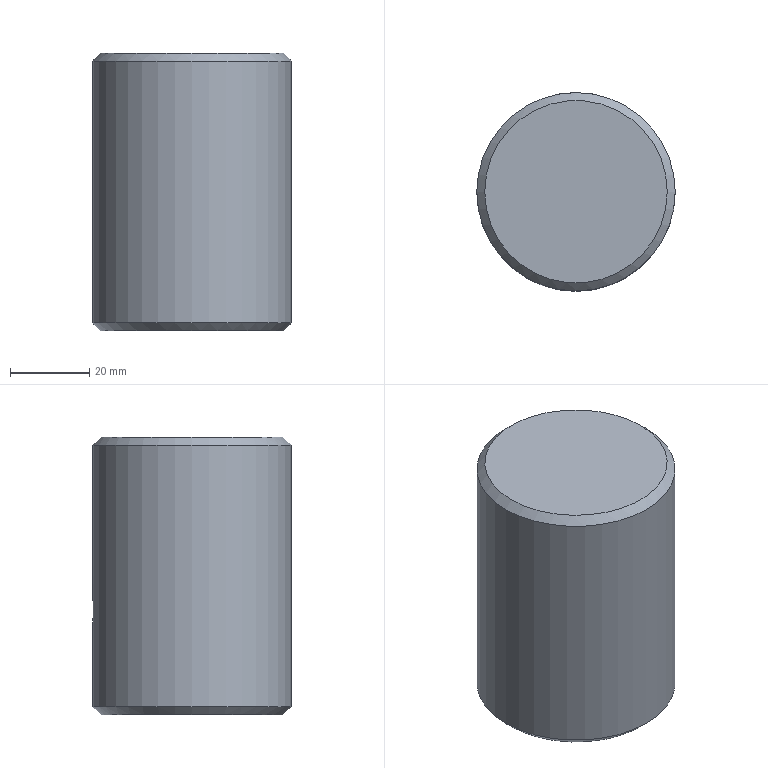Part | NX | features LIN_SOLID_COLOR 2 | 1 solid | 9 faces | box 50 x 50 x 70 mm | volume 134795 mm3 | cone 4 | cylinder 3 | plane 2 | commonest cylinder face diameters 5.2 x1 8.499 x1 50 x1
STEP:
#1=CARTESIAN_POINT('',(609.,370.,-46.5));
#2=VERTEX_POINT('',#1);
#3=CARTESIAN_POINT('',(586.,370.,-46.5));
#4=DIRECTION('',(0.,0.,-1.));
#5=DIRECTION('',(1.,0.,0.));
#6=AXIS2_PLACEMENT_3D('',#3,#4,#5);
#7=CIRCLE('',#6,23.);
#8=EDGE_CURVE('',#2,#2,#7,.T.);
#9=ORIENTED_EDGE('',*,*,#8,.T.);
#10=EDGE_LOOP('',(#9));
#11=FACE_BOUND('',#10,.T.);
#12=CARTESIAN_POINT('',(590.25,370.,-46.5));
#13=VERTEX_POINT('',#12);
#14=CARTESIAN_POINT('',(586.,370.,-46.5));
#15=DIRECTION('',(0.,0.,1.));
#16=DIRECTION('',(1.,0.,0.));
#17=AXIS2_PLACEMENT_3D('',#14,#15,#16);
#18=CIRCLE('',#17,4.25);
#19=EDGE_CURVE('',#13,#13,#18,.T.);
#20=ORIENTED_EDGE('',*,*,#19,.T.);
#21=EDGE_LOOP('',(#20));
#22=FACE_BOUND('',#21,.T.);
#23=CARTESIAN_POINT('',(586.,370.,-46.5));
#24=DIRECTION('',(0.,0.,-1.));
#25=DIRECTION('',(1.,0.,0.));
#26=AXIS2_PLACEMENT_3D('',#23,#24,#25);
#27=PLANE('',#26);
#28=ADVANCED_FACE('',(#11,#22),#27,.T.);
#29=CARTESIAN_POINT('',(563.,370.,23.5));
#30=VERTEX_POINT('',#29);
#31=CARTESIAN_POINT('',(586.,370.,23.5));
#32=DIRECTION('',(0.,0.,1.));
#33=DIRECTION('',(-1.,0.,0.));
#34=AXIS2_PLACEMENT_3D('',#31,#32,#33);
#35=CIRCLE('',#34,23.);
#36=EDGE_CURVE('',#30,#30,#35,.T.);
#37=ORIENTED_EDGE('',*,*,#36,.T.);
#38=EDGE_LOOP('',(#37));
#39=FACE_BOUND('',#38,.T.);
#40=CARTESIAN_POINT('',(586.,370.,23.5));
#41=DIRECTION('',(0.,0.,1.));
#42=DIRECTION('',(-1.,0.,0.));
#43=AXIS2_PLACEMENT_3D('',#40,#41,#42);
#44=PLANE('',#43);
#45=ADVANCED_FACE('',(#39),#44,.T.);
#46=CARTESIAN_POINT('',(588.6,394.864,-20.));
#47=VERTEX_POINT('',#46);
#48=CARTESIAN_POINT('',(588.036,394.933,-17.96));
#49=CARTESIAN_POINT('',(588.882,394.83,-20.001));
#50=CARTESIAN_POINT('',(588.036,394.932,-22.038));
#51=CARTESIAN_POINT('',(586.002,395.034,-22.881));
#52=CARTESIAN_POINT('',(583.963,394.932,-22.039));
#53=CARTESIAN_POINT('',(583.119,394.83,-20.001));
#54=CARTESIAN_POINT('',(583.961,394.932,-17.965));
#55=CARTESIAN_POINT('',(585.997,395.034,-17.119));
#56=CARTESIAN_POINT('',(588.036,394.933,-17.96));
#57=CARTESIAN_POINT('',(588.882,394.83,-20.001));
#58=CARTESIAN_POINT('',(588.036,394.932,-22.038));
#59=B_SPLINE_CURVE_WITH_KNOTS('',3,(#48,#49,#50,#51,#52,#53,#54,#55,#56,#57,#58),.UNSPECIFIED.,.T.,.F.,(1,1,1,1,1,1,1,1,1,1,1,1,1,1,1),(-0.0061,-0.004067,-0.002033,0.,0.002033,0.004067,0.0061,0.008133,0.01017,0.0122,0.01423,0.01627,0.0183,0.02033,0.02237),.UNSPECIFIED.);
#60=EDGE_CURVE('',#47,#47,#59,.T.);
#61=ORIENTED_EDGE('',*,*,#60,.F.);
#62=EDGE_LOOP('',(#61));
#63=FACE_BOUND('',#62,.T.);
#64=CARTESIAN_POINT('',(611.,370.,-44.5));
#65=VERTEX_POINT('',#64);
#66=CARTESIAN_POINT('',(586.,370.,-44.5));
#67=DIRECTION('',(0.,0.,-1.));
#68=DIRECTION('',(1.,0.,0.));
#69=AXIS2_PLACEMENT_3D('',#66,#67,#68);
#70=CIRCLE('',#69,25.);
#71=EDGE_CURVE('',#65,#65,#70,.F.);
#72=ORIENTED_EDGE('',*,*,#71,.T.);
#73=EDGE_LOOP('',(#72));
#74=FACE_BOUND('',#73,.T.);
#75=CARTESIAN_POINT('',(561.,370.,21.5));
#76=VERTEX_POINT('',#75);
#77=CARTESIAN_POINT('',(586.,370.,21.5));
#78=DIRECTION('',(0.,0.,1.));
#79=DIRECTION('',(-1.,0.,0.));
#80=AXIS2_PLACEMENT_3D('',#77,#78,#79);
#81=CIRCLE('',#80,25.);
#82=EDGE_CURVE('',#76,#76,#81,.F.);
#83=ORIENTED_EDGE('',*,*,#82,.T.);
#84=EDGE_LOOP('',(#83));
#85=FACE_BOUND('',#84,.T.);
#86=CARTESIAN_POINT('',(586.,370.,3.5));
#87=DIRECTION('',(0.,0.,-1.));
#88=DIRECTION('',(1.,0.,0.));
#89=AXIS2_PLACEMENT_3D('',#86,#87,#88);
#90=CYLINDRICAL_SURFACE('',#89,25.);
#91=ADVANCED_FACE('',(#63,#74,#85),#90,.T.);
#92=ORIENTED_EDGE('',*,*,#71,.F.);
#93=EDGE_LOOP('',(#92));
#94=FACE_BOUND('',#93,.T.);
#95=ORIENTED_EDGE('',*,*,#8,.F.);
#96=EDGE_LOOP('',(#95));
#97=FACE_BOUND('',#96,.T.);
#98=CARTESIAN_POINT('',(586.,370.,-46.5));
#99=DIRECTION('',(0.,0.,1.));
#100=DIRECTION('',(-1.,0.,0.));
#101=AXIS2_PLACEMENT_3D('',#98,#99,#100);
#102=CONICAL_SURFACE('',#101,23.,0.7854);
#103=ADVANCED_FACE('',(#94,#97),#102,.T.);
#104=ORIENTED_EDGE('',*,*,#36,.F.);
#105=EDGE_LOOP('',(#104));
#106=FACE_BOUND('',#105,.T.);
#107=ORIENTED_EDGE('',*,*,#82,.F.);
#108=EDGE_LOOP('',(#107));
#109=FACE_BOUND('',#108,.T.);
#110=CARTESIAN_POINT('',(586.,370.,21.5));
#111=DIRECTION('',(0.,0.,-1.));
#112=DIRECTION('',(1.,0.,0.));
#113=AXIS2_PLACEMENT_3D('',#110,#111,#112);
#114=CONICAL_SURFACE('',#113,25.,0.7854);
#115=ADVANCED_FACE('',(#106,#109),#114,.T.);
#116=ORIENTED_EDGE('',*,*,#60,.T.);
#117=EDGE_LOOP('',(#116));
#118=FACE_BOUND('',#117,.T.);
#119=CARTESIAN_POINT('',(583.4,383.1,-20.));
#120=VERTEX_POINT('',#119);
#121=CARTESIAN_POINT('',(586.,383.1,-20.));
#122=DIRECTION('',(0.,-1.,0.));
#123=DIRECTION('',(-1.,0.,0.));
#124=AXIS2_PLACEMENT_3D('',#121,#122,#123);
#125=CIRCLE('',#124,2.6);
#126=EDGE_CURVE('',#120,#120,#125,.T.);
#127=ORIENTED_EDGE('',*,*,#126,.T.);
#128=EDGE_LOOP('',(#127));
#129=FACE_BOUND('',#128,.T.);
#130=CARTESIAN_POINT('',(586.,404.5,-20.));
#131=DIRECTION('',(0.,-1.,0.));
#132=DIRECTION('',(1.,0.,0.));
#133=AXIS2_PLACEMENT_3D('',#130,#131,#132);
#134=CYLINDRICAL_SURFACE('',#133,2.6);
#135=ADVANCED_FACE('',(#118,#129),#134,.F.);
#136=CARTESIAN_POINT('',(586.,380.5,-20.));
#137=VERTEX_POINT('',#136);
#138=VERTEX_LOOP('',#137);
#139=FACE_BOUND('',#138,.T.);
#140=ORIENTED_EDGE('',*,*,#126,.F.);
#141=EDGE_LOOP('',(#140));
#142=FACE_BOUND('',#141,.T.);
#143=CARTESIAN_POINT('',(586.,383.1,-20.));
#144=DIRECTION('',(0.,1.,0.));
#145=DIRECTION('',(1.,0.,0.));
#146=AXIS2_PLACEMENT_3D('',#143,#144,#145);
#147=CONICAL_SURFACE('',#146,2.6,0.7854);
#148=ADVANCED_FACE('',(#139,#142),#147,.F.);
#149=CARTESIAN_POINT('',(590.25,370.,-16.75));
#150=VERTEX_POINT('',#149);
#151=CARTESIAN_POINT('',(586.,370.,-16.75));
#152=DIRECTION('',(0.,0.,1.));
#153=DIRECTION('',(1.,0.,0.));
#154=AXIS2_PLACEMENT_3D('',#151,#152,#153);
#155=CIRCLE('',#154,4.25);
#156=EDGE_CURVE('',#150,#150,#155,.T.);
#157=ORIENTED_EDGE('',*,*,#156,.T.);
#158=EDGE_LOOP('',(#157));
#159=FACE_BOUND('',#158,.T.);
#160=ORIENTED_EDGE('',*,*,#19,.F.);
#161=EDGE_LOOP('',(#160));
#162=FACE_BOUND('',#161,.T.);
#163=CARTESIAN_POINT('',(586.,370.,-46.5));
#164=DIRECTION('',(0.,0.,1.));
#165=DIRECTION('',(1.,0.,0.));
#166=AXIS2_PLACEMENT_3D('',#163,#164,#165);
#167=CYLINDRICAL_SURFACE('',#166,4.25);
#168=ADVANCED_FACE('',(#159,#162),#167,.F.);
#169=CARTESIAN_POINT('',(586.,370.,-12.5));
#170=VERTEX_POINT('',#169);
#171=VERTEX_LOOP('',#170);
#172=FACE_BOUND('',#171,.T.);
#173=ORIENTED_EDGE('',*,*,#156,.F.);
#174=EDGE_LOOP('',(#173));
#175=FACE_BOUND('',#174,.T.);
#176=CARTESIAN_POINT('',(586.,370.,-16.75));
#177=DIRECTION('',(0.,0.,-1.));
#178=DIRECTION('',(-1.,0.,0.));
#179=AXIS2_PLACEMENT_3D('',#176,#177,#178);
#180=CONICAL_SURFACE('',#179,4.25,0.7854);
#181=ADVANCED_FACE('',(#172,#175),#180,.F.);
#182=CLOSED_SHELL('',(#28,#45,#91,#103,#115,#135,#148,#168,#181));
#183=MANIFOLD_SOLID_BREP('',#182);
#184=(LENGTH_UNIT()NAMED_UNIT(*)SI_UNIT(.MILLI.,.METRE.));
#185=UNCERTAINTY_MEASURE_WITH_UNIT(LENGTH_MEASURE(0.0508),#184,'','');
#186=(NAMED_UNIT(*)PLANE_ANGLE_UNIT()SI_UNIT($,.RADIAN.));
#187=(NAMED_UNIT(*)SI_UNIT($,.STERADIAN.)SOLID_ANGLE_UNIT());
#188=(GEOMETRIC_REPRESENTATION_CONTEXT(3)GLOBAL_UNCERTAINTY_ASSIGNED_CONTEXT((#185))GLOBAL_UNIT_ASSIGNED_CONTEXT((#184,#186,#187))REPRESENTATION_CONTEXT('',''));
#189=ADVANCED_BREP_SHAPE_REPRESENTATION('',(#183),#188);